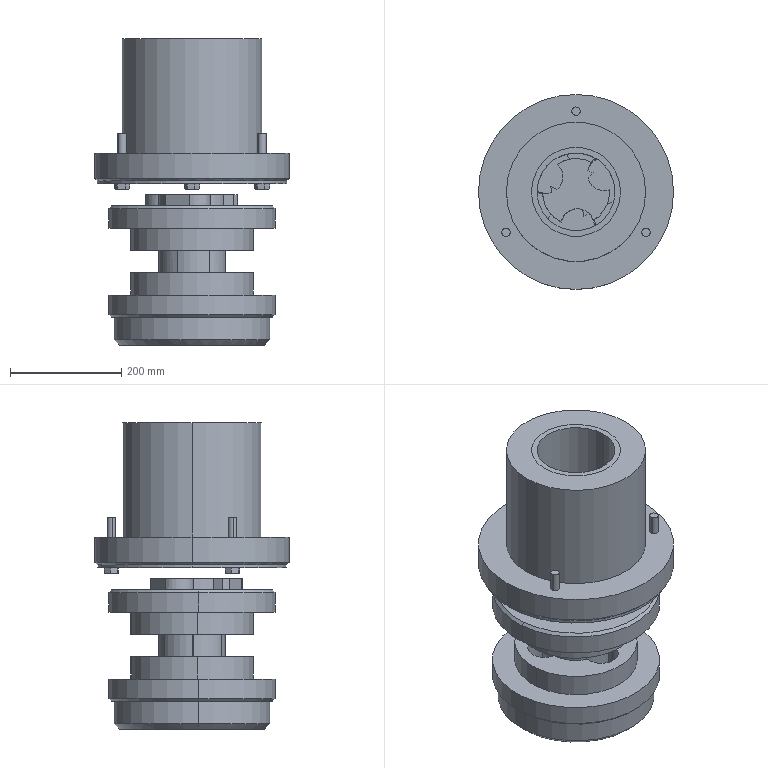Part | SolidWorks | 13 solids | 213 faces | box 350 x 350 x 550 mm | volume 23094575 mm3 | cylinder 98 | plane 83 | cone 32 | commonest cylinder face diameters 120 x30 60 x20 15 x18 220 x6 140 x4 160 x4